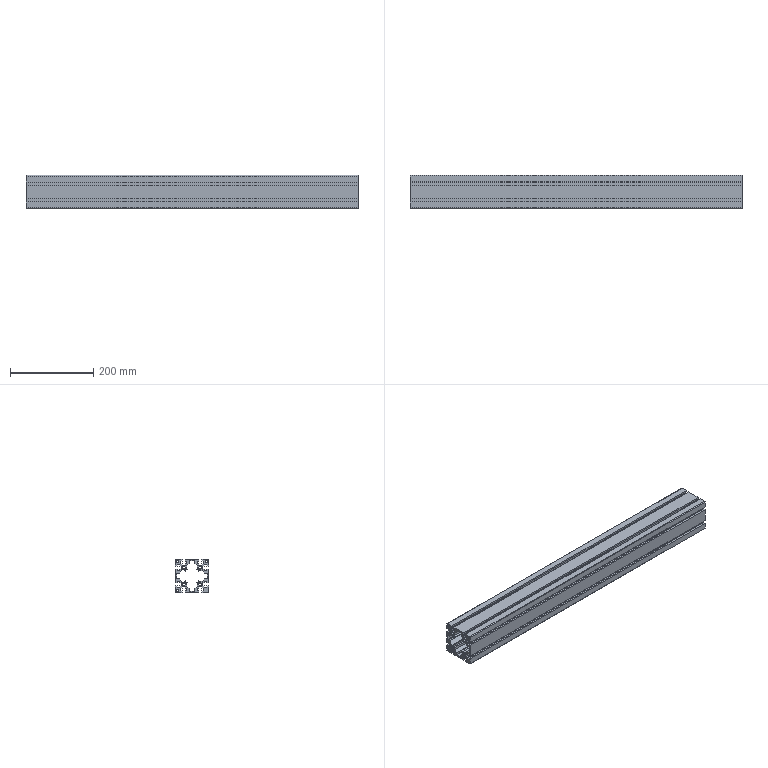Part | NX | 1 solid | 165 faces | box 800 x 80 x 80 mm | volume 1853836 mm3 | plane 146 | cylinder 19 | commonest cylinder face diameters 2 x8 3 x4 6.8 x4 6 x3